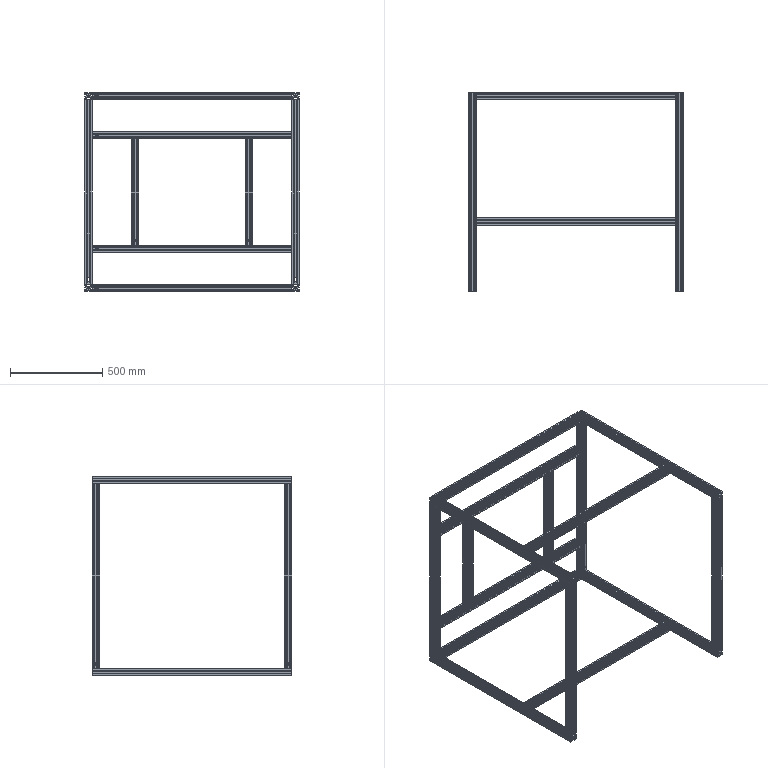Part | SolidWorks | 16 solids | 1184 faces | box 1160 x 1080 x 1080 mm | volume 12576449 mm3 | plane 964 | cylinder 220 | commonest cylinder face diameters 6 x128 20.5 x60 10.5 x32